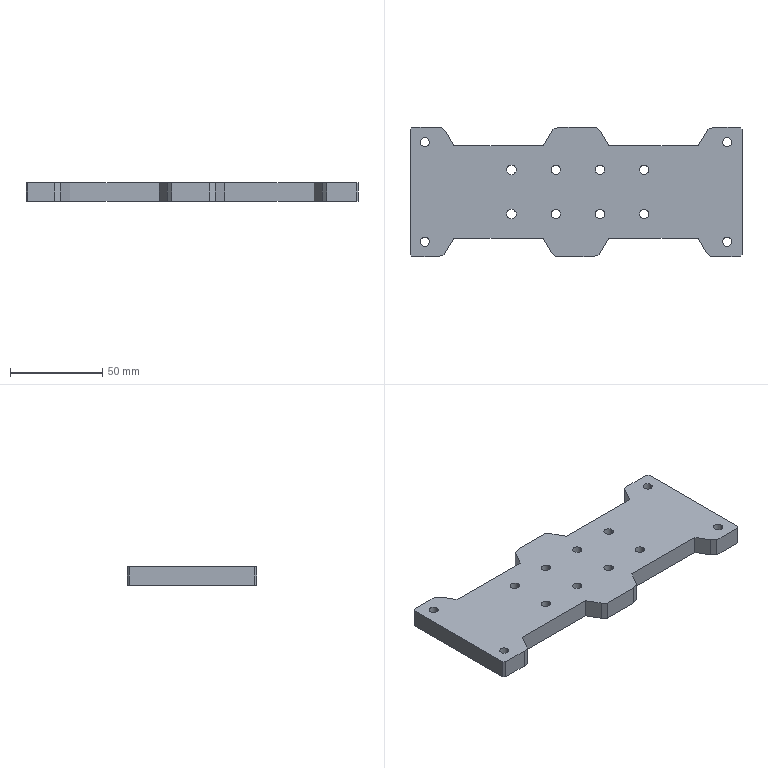Part | SolidWorks | features ICE 3, Chamfer 1, Extrusion 1 | 1 solid | 58 faces | box 180 x 70 x 10 mm | volume 101775 mm3 | plane 34 | cylinder 24 | commonest cylinder face diameters 5.1 x16 5 x8